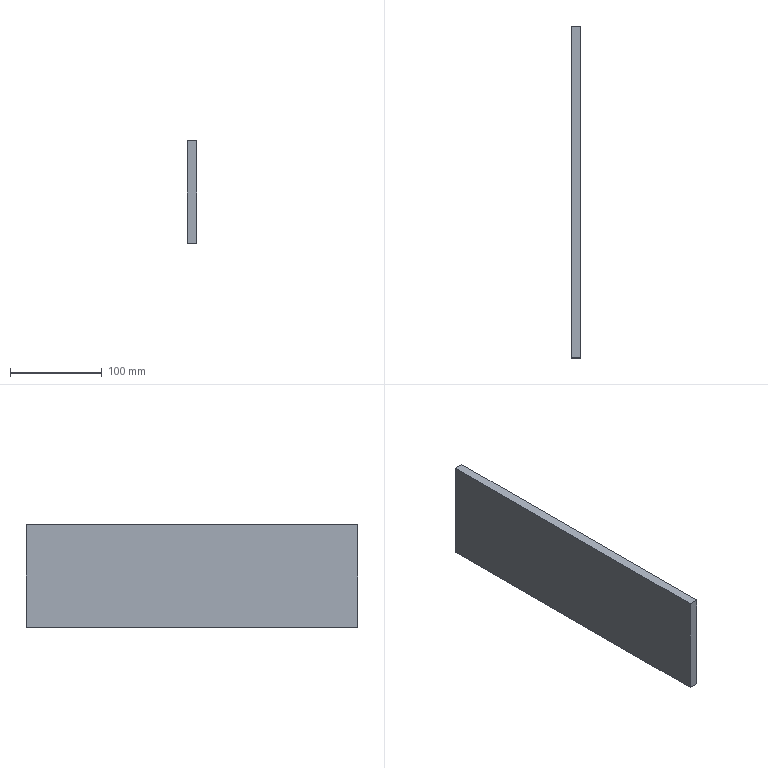Part | STEP file | Drawer | 1 solid | 6 faces | box 10 x 362 x 112 mm | volume 405440 mm3 | plane 6
STEP:
#1=CARTESIAN_POINT('',(0.,0.,0.));
#2=DIRECTION('',(0.,0.,1.));
#3=DIRECTION('',(1.,0.,0.));
#4=AXIS2_PLACEMENT_3D('',#1,#2,#3);
#5=CARTESIAN_POINT('',(-5.,181.,112.));
#6=VERTEX_POINT('',#5);
#7=CARTESIAN_POINT('',(-5.,-181.,112.));
#8=VERTEX_POINT('',#7);
#9=CARTESIAN_POINT('',(-5.,181.,112.));
#10=DIRECTION('',(0.,-1.,0.));
#11=VECTOR('',#10,1.);
#12=LINE('',#9,#11);
#13=CARTESIAN_POINT('',(-5.,181.,112.));
#14=DIRECTION('',(1.,0.,0.));
#15=DIRECTION('',(0.,0.,-1.));
#16=AXIS2_PLACEMENT_3D('',#13,#14,#15);
#17=PLANE('',#16);
#18=CARTESIAN_POINT('',(0.,0.));
#19=DIRECTION('',(0.,-1.));
#20=VECTOR('',#19,1.);
#21=LINE('',#18,#20);
#22=(GEOMETRIC_REPRESENTATION_CONTEXT(2)PARAMETRIC_REPRESENTATION_CONTEXT()REPRESENTATION_CONTEXT('',''));
#23=DEFINITIONAL_REPRESENTATION('',(#21),#22);
#24=PCURVE('',#17,#23);
#25=CARTESIAN_POINT('',(5.,181.,112.));
#26=DIRECTION('',(0.,0.,-1.));
#27=DIRECTION('',(-1.,0.,0.));
#28=AXIS2_PLACEMENT_3D('',#25,#26,#27);
#29=PLANE('',#28);
#30=CARTESIAN_POINT('',(10.,0.));
#31=DIRECTION('',(0.,-1.));
#32=VECTOR('',#31,1.);
#33=LINE('',#30,#32);
#34=(GEOMETRIC_REPRESENTATION_CONTEXT(2)PARAMETRIC_REPRESENTATION_CONTEXT()REPRESENTATION_CONTEXT('',''));
#35=DEFINITIONAL_REPRESENTATION('',(#33),#34);
#36=PCURVE('',#29,#35);
#37=SURFACE_CURVE('',#12,(#24,#36),.PCURVE_S1.);
#38=EDGE_CURVE('',#6,#8,#37,.T.);
#39=ORIENTED_EDGE('',*,*,#38,.T.);
#40=CARTESIAN_POINT('',(-5.,-181.,0.));
#41=VERTEX_POINT('',#40);
#42=CARTESIAN_POINT('',(-5.,-181.,112.));
#43=DIRECTION('',(0.,0.,-1.));
#44=VECTOR('',#43,1.);
#45=LINE('',#42,#44);
#46=CARTESIAN_POINT('',(0.,-362.));
#47=DIRECTION('',(1.,0.));
#48=VECTOR('',#47,1.);
#49=LINE('',#46,#48);
#50=(GEOMETRIC_REPRESENTATION_CONTEXT(2)PARAMETRIC_REPRESENTATION_CONTEXT()REPRESENTATION_CONTEXT('',''));
#51=DEFINITIONAL_REPRESENTATION('',(#49),#50);
#52=PCURVE('',#17,#51);
#53=CARTESIAN_POINT('',(0.,-181.,56.));
#54=DIRECTION('',(0.,1.,0.));
#55=DIRECTION('',(0.,0.,1.));
#56=AXIS2_PLACEMENT_3D('',#53,#54,#55);
#57=PLANE('',#56);
#58=CARTESIAN_POINT('',(56.,-5.));
#59=DIRECTION('',(-1.,0.));
#60=VECTOR('',#59,1.);
#61=LINE('',#58,#60);
#62=(GEOMETRIC_REPRESENTATION_CONTEXT(2)PARAMETRIC_REPRESENTATION_CONTEXT()REPRESENTATION_CONTEXT('',''));
#63=DEFINITIONAL_REPRESENTATION('',(#61),#62);
#64=PCURVE('',#57,#63);
#65=SURFACE_CURVE('',#45,(#52,#64),.PCURVE_S1.);
#66=EDGE_CURVE('',#8,#41,#65,.T.);
#67=ORIENTED_EDGE('',*,*,#66,.T.);
#68=CARTESIAN_POINT('',(-5.,181.,0.));
#69=VERTEX_POINT('',#68);
#70=CARTESIAN_POINT('',(-5.,181.,0.));
#71=DIRECTION('',(0.,-1.,0.));
#72=VECTOR('',#71,1.);
#73=LINE('',#70,#72);
#74=CARTESIAN_POINT('',(112.,0.));
#75=DIRECTION('',(0.,-1.));
#76=VECTOR('',#75,1.);
#77=LINE('',#74,#76);
#78=(GEOMETRIC_REPRESENTATION_CONTEXT(2)PARAMETRIC_REPRESENTATION_CONTEXT()REPRESENTATION_CONTEXT('',''));
#79=DEFINITIONAL_REPRESENTATION('',(#77),#78);
#80=PCURVE('',#17,#79);
#81=CARTESIAN_POINT('',(-5.,181.,0.));
#82=DIRECTION('',(0.,0.,1.));
#83=DIRECTION('',(1.,0.,0.));
#84=AXIS2_PLACEMENT_3D('',#81,#82,#83);
#85=PLANE('',#84);
#86=CARTESIAN_POINT('',(0.,0.));
#87=DIRECTION('',(0.,-1.));
#88=VECTOR('',#87,1.);
#89=LINE('',#86,#88);
#90=(GEOMETRIC_REPRESENTATION_CONTEXT(2)PARAMETRIC_REPRESENTATION_CONTEXT()REPRESENTATION_CONTEXT('',''));
#91=DEFINITIONAL_REPRESENTATION('',(#89),#90);
#92=PCURVE('',#85,#91);
#93=SURFACE_CURVE('',#73,(#80,#92),.PCURVE_S1.);
#94=EDGE_CURVE('',#69,#41,#93,.T.);
#95=ORIENTED_EDGE('',*,*,#94,.F.);
#96=CARTESIAN_POINT('',(-5.,181.,112.));
#97=DIRECTION('',(0.,0.,-1.));
#98=VECTOR('',#97,1.);
#99=LINE('',#96,#98);
#100=CARTESIAN_POINT('',(0.,0.));
#101=DIRECTION('',(1.,0.));
#102=VECTOR('',#101,1.);
#103=LINE('',#100,#102);
#104=(GEOMETRIC_REPRESENTATION_CONTEXT(2)PARAMETRIC_REPRESENTATION_CONTEXT()REPRESENTATION_CONTEXT('',''));
#105=DEFINITIONAL_REPRESENTATION('',(#103),#104);
#106=PCURVE('',#17,#105);
#107=CARTESIAN_POINT('',(0.,181.,56.));
#108=DIRECTION('',(0.,1.,0.));
#109=DIRECTION('',(0.,0.,1.));
#110=AXIS2_PLACEMENT_3D('',#107,#108,#109);
#111=PLANE('',#110);
#112=CARTESIAN_POINT('',(56.,-5.));
#113=DIRECTION('',(-1.,0.));
#114=VECTOR('',#113,1.);
#115=LINE('',#112,#114);
#116=(GEOMETRIC_REPRESENTATION_CONTEXT(2)PARAMETRIC_REPRESENTATION_CONTEXT()REPRESENTATION_CONTEXT('',''));
#117=DEFINITIONAL_REPRESENTATION('',(#115),#116);
#118=PCURVE('',#111,#117);
#119=SURFACE_CURVE('',#99,(#106,#118),.PCURVE_S1.);
#120=EDGE_CURVE('',#6,#69,#119,.T.);
#121=ORIENTED_EDGE('',*,*,#120,.F.);
#122=EDGE_LOOP('',(#39,#67,#95,#121));
#123=FACE_BOUND('',#122,.F.);
#124=ADVANCED_FACE('',(#123),#17,.F.);
#125=ORIENTED_EDGE('',*,*,#94,.T.);
#126=CARTESIAN_POINT('',(5.,-181.,0.));
#127=VERTEX_POINT('',#126);
#128=CARTESIAN_POINT('',(-5.,-181.,0.));
#129=DIRECTION('',(1.,0.,0.));
#130=VECTOR('',#129,1.);
#131=LINE('',#128,#130);
#132=CARTESIAN_POINT('',(0.,-362.));
#133=DIRECTION('',(1.,0.));
#134=VECTOR('',#133,1.);
#135=LINE('',#132,#134);
#136=(GEOMETRIC_REPRESENTATION_CONTEXT(2)PARAMETRIC_REPRESENTATION_CONTEXT()REPRESENTATION_CONTEXT('',''));
#137=DEFINITIONAL_REPRESENTATION('',(#135),#136);
#138=PCURVE('',#85,#137);
#139=CARTESIAN_POINT('',(-56.,-5.));
#140=DIRECTION('',(0.,1.));
#141=VECTOR('',#140,1.);
#142=LINE('',#139,#141);
#143=(GEOMETRIC_REPRESENTATION_CONTEXT(2)PARAMETRIC_REPRESENTATION_CONTEXT()REPRESENTATION_CONTEXT('',''));
#144=DEFINITIONAL_REPRESENTATION('',(#142),#143);
#145=PCURVE('',#57,#144);
#146=SURFACE_CURVE('',#131,(#138,#145),.PCURVE_S1.);
#147=EDGE_CURVE('',#41,#127,#146,.T.);
#148=ORIENTED_EDGE('',*,*,#147,.T.);
#149=CARTESIAN_POINT('',(5.,181.,0.));
#150=VERTEX_POINT('',#149);
#151=CARTESIAN_POINT('',(5.,181.,0.));
#152=DIRECTION('',(0.,-1.,0.));
#153=VECTOR('',#152,1.);
#154=LINE('',#151,#153);
#155=CARTESIAN_POINT('',(10.,0.));
#156=DIRECTION('',(0.,-1.));
#157=VECTOR('',#156,1.);
#158=LINE('',#155,#157);
#159=(GEOMETRIC_REPRESENTATION_CONTEXT(2)PARAMETRIC_REPRESENTATION_CONTEXT()REPRESENTATION_CONTEXT('',''));
#160=DEFINITIONAL_REPRESENTATION('',(#158),#159);
#161=PCURVE('',#85,#160);
#162=CARTESIAN_POINT('',(5.,181.,0.));
#163=DIRECTION('',(-1.,0.,0.));
#164=DIRECTION('',(0.,0.,1.));
#165=AXIS2_PLACEMENT_3D('',#162,#163,#164);
#166=PLANE('',#165);
#167=CARTESIAN_POINT('',(0.,0.));
#168=DIRECTION('',(0.,-1.));
#169=VECTOR('',#168,1.);
#170=LINE('',#167,#169);
#171=(GEOMETRIC_REPRESENTATION_CONTEXT(2)PARAMETRIC_REPRESENTATION_CONTEXT()REPRESENTATION_CONTEXT('',''));
#172=DEFINITIONAL_REPRESENTATION('',(#170),#171);
#173=PCURVE('',#166,#172);
#174=SURFACE_CURVE('',#154,(#161,#173),.PCURVE_S1.);
#175=EDGE_CURVE('',#150,#127,#174,.T.);
#176=ORIENTED_EDGE('',*,*,#175,.F.);
#177=CARTESIAN_POINT('',(-5.,181.,0.));
#178=DIRECTION('',(1.,0.,0.));
#179=VECTOR('',#178,1.);
#180=LINE('',#177,#179);
#181=CARTESIAN_POINT('',(0.,0.));
#182=DIRECTION('',(1.,0.));
#183=VECTOR('',#182,1.);
#184=LINE('',#181,#183);
#185=(GEOMETRIC_REPRESENTATION_CONTEXT(2)PARAMETRIC_REPRESENTATION_CONTEXT()REPRESENTATION_CONTEXT('',''));
#186=DEFINITIONAL_REPRESENTATION('',(#184),#185);
#187=PCURVE('',#85,#186);
#188=CARTESIAN_POINT('',(-56.,-5.));
#189=DIRECTION('',(0.,1.));
#190=VECTOR('',#189,1.);
#191=LINE('',#188,#190);
#192=(GEOMETRIC_REPRESENTATION_CONTEXT(2)PARAMETRIC_REPRESENTATION_CONTEXT()REPRESENTATION_CONTEXT('',''));
#193=DEFINITIONAL_REPRESENTATION('',(#191),#192);
#194=PCURVE('',#111,#193);
#195=SURFACE_CURVE('',#180,(#187,#194),.PCURVE_S1.);
#196=EDGE_CURVE('',#69,#150,#195,.T.);
#197=ORIENTED_EDGE('',*,*,#196,.F.);
#198=EDGE_LOOP('',(#125,#148,#176,#197));
#199=FACE_BOUND('',#198,.F.);
#200=ADVANCED_FACE('',(#199),#85,.F.);
#201=ORIENTED_EDGE('',*,*,#175,.T.);
#202=CARTESIAN_POINT('',(5.,-181.,112.));
#203=VERTEX_POINT('',#202);
#204=CARTESIAN_POINT('',(5.,-181.,0.));
#205=DIRECTION('',(0.,0.,1.));
#206=VECTOR('',#205,1.);
#207=LINE('',#204,#206);
#208=CARTESIAN_POINT('',(0.,-362.));
#209=DIRECTION('',(1.,0.));
#210=VECTOR('',#209,1.);
#211=LINE('',#208,#210);
#212=(GEOMETRIC_REPRESENTATION_CONTEXT(2)PARAMETRIC_REPRESENTATION_CONTEXT()REPRESENTATION_CONTEXT('',''));
#213=DEFINITIONAL_REPRESENTATION('',(#211),#212);
#214=PCURVE('',#166,#213);
#215=CARTESIAN_POINT('',(-56.,5.));
#216=DIRECTION('',(1.,0.));
#217=VECTOR('',#216,1.);
#218=LINE('',#215,#217);
#219=(GEOMETRIC_REPRESENTATION_CONTEXT(2)PARAMETRIC_REPRESENTATION_CONTEXT()REPRESENTATION_CONTEXT('',''));
#220=DEFINITIONAL_REPRESENTATION('',(#218),#219);
#221=PCURVE('',#57,#220);
#222=SURFACE_CURVE('',#207,(#214,#221),.PCURVE_S1.);
#223=EDGE_CURVE('',#127,#203,#222,.T.);
#224=ORIENTED_EDGE('',*,*,#223,.T.);
#225=CARTESIAN_POINT('',(5.,181.,112.));
#226=VERTEX_POINT('',#225);
#227=CARTESIAN_POINT('',(5.,181.,112.));
#228=DIRECTION('',(0.,-1.,0.));
#229=VECTOR('',#228,1.);
#230=LINE('',#227,#229);
#231=CARTESIAN_POINT('',(112.,0.));
#232=DIRECTION('',(0.,-1.));
#233=VECTOR('',#232,1.);
#234=LINE('',#231,#233);
#235=(GEOMETRIC_REPRESENTATION_CONTEXT(2)PARAMETRIC_REPRESENTATION_CONTEXT()REPRESENTATION_CONTEXT('',''));
#236=DEFINITIONAL_REPRESENTATION('',(#234),#235);
#237=PCURVE('',#166,#236);
#238=CARTESIAN_POINT('',(0.,0.));
#239=DIRECTION('',(0.,-1.));
#240=VECTOR('',#239,1.);
#241=LINE('',#238,#240);
#242=(GEOMETRIC_REPRESENTATION_CONTEXT(2)PARAMETRIC_REPRESENTATION_CONTEXT()REPRESENTATION_CONTEXT('',''));
#243=DEFINITIONAL_REPRESENTATION('',(#241),#242);
#244=PCURVE('',#29,#243);
#245=SURFACE_CURVE('',#230,(#237,#244),.PCURVE_S1.);
#246=EDGE_CURVE('',#226,#203,#245,.T.);
#247=ORIENTED_EDGE('',*,*,#246,.F.);
#248=CARTESIAN_POINT('',(5.,181.,0.));
#249=DIRECTION('',(0.,0.,1.));
#250=VECTOR('',#249,1.);
#251=LINE('',#248,#250);
#252=CARTESIAN_POINT('',(0.,0.));
#253=DIRECTION('',(1.,0.));
#254=VECTOR('',#253,1.);
#255=LINE('',#252,#254);
#256=(GEOMETRIC_REPRESENTATION_CONTEXT(2)PARAMETRIC_REPRESENTATION_CONTEXT()REPRESENTATION_CONTEXT('',''));
#257=DEFINITIONAL_REPRESENTATION('',(#255),#256);
#258=PCURVE('',#166,#257);
#259=CARTESIAN_POINT('',(-56.,5.));
#260=DIRECTION('',(1.,0.));
#261=VECTOR('',#260,1.);
#262=LINE('',#259,#261);
#263=(GEOMETRIC_REPRESENTATION_CONTEXT(2)PARAMETRIC_REPRESENTATION_CONTEXT()REPRESENTATION_CONTEXT('',''));
#264=DEFINITIONAL_REPRESENTATION('',(#262),#263);
#265=PCURVE('',#111,#264);
#266=SURFACE_CURVE('',#251,(#258,#265),.PCURVE_S1.);
#267=EDGE_CURVE('',#150,#226,#266,.T.);
#268=ORIENTED_EDGE('',*,*,#267,.F.);
#269=EDGE_LOOP('',(#201,#224,#247,#268));
#270=FACE_BOUND('',#269,.F.);
#271=ADVANCED_FACE('',(#270),#166,.F.);
#272=ORIENTED_EDGE('',*,*,#246,.T.);
#273=CARTESIAN_POINT('',(5.,-181.,112.));
#274=DIRECTION('',(-1.,0.,0.));
#275=VECTOR('',#274,1.);
#276=LINE('',#273,#275);
#277=CARTESIAN_POINT('',(0.,-362.));
#278=DIRECTION('',(1.,0.));
#279=VECTOR('',#278,1.);
#280=LINE('',#277,#279);
#281=(GEOMETRIC_REPRESENTATION_CONTEXT(2)PARAMETRIC_REPRESENTATION_CONTEXT()REPRESENTATION_CONTEXT('',''));
#282=DEFINITIONAL_REPRESENTATION('',(#280),#281);
#283=PCURVE('',#29,#282);
#284=CARTESIAN_POINT('',(56.,5.));
#285=DIRECTION('',(0.,-1.));
#286=VECTOR('',#285,1.);
#287=LINE('',#284,#286);
#288=(GEOMETRIC_REPRESENTATION_CONTEXT(2)PARAMETRIC_REPRESENTATION_CONTEXT()REPRESENTATION_CONTEXT('',''));
#289=DEFINITIONAL_REPRESENTATION('',(#287),#288);
#290=PCURVE('',#57,#289);
#291=SURFACE_CURVE('',#276,(#283,#290),.PCURVE_S1.);
#292=EDGE_CURVE('',#203,#8,#291,.T.);
#293=ORIENTED_EDGE('',*,*,#292,.T.);
#294=ORIENTED_EDGE('',*,*,#38,.F.);
#295=CARTESIAN_POINT('',(5.,181.,112.));
#296=DIRECTION('',(-1.,0.,0.));
#297=VECTOR('',#296,1.);
#298=LINE('',#295,#297);
#299=CARTESIAN_POINT('',(0.,0.));
#300=DIRECTION('',(1.,0.));
#301=VECTOR('',#300,1.);
#302=LINE('',#299,#301);
#303=(GEOMETRIC_REPRESENTATION_CONTEXT(2)PARAMETRIC_REPRESENTATION_CONTEXT()REPRESENTATION_CONTEXT('',''));
#304=DEFINITIONAL_REPRESENTATION('',(#302),#303);
#305=PCURVE('',#29,#304);
#306=CARTESIAN_POINT('',(56.,5.));
#307=DIRECTION('',(0.,-1.));
#308=VECTOR('',#307,1.);
#309=LINE('',#306,#308);
#310=(GEOMETRIC_REPRESENTATION_CONTEXT(2)PARAMETRIC_REPRESENTATION_CONTEXT()REPRESENTATION_CONTEXT('',''));
#311=DEFINITIONAL_REPRESENTATION('',(#309),#310);
#312=PCURVE('',#111,#311);
#313=SURFACE_CURVE('',#298,(#305,#312),.PCURVE_S1.);
#314=EDGE_CURVE('',#226,#6,#313,.T.);
#315=ORIENTED_EDGE('',*,*,#314,.F.);
#316=EDGE_LOOP('',(#272,#293,#294,#315));
#317=FACE_BOUND('',#316,.F.);
#318=ADVANCED_FACE('',(#317),#29,.F.);
#319=ORIENTED_EDGE('',*,*,#120,.T.);
#320=ORIENTED_EDGE('',*,*,#196,.T.);
#321=ORIENTED_EDGE('',*,*,#267,.T.);
#322=ORIENTED_EDGE('',*,*,#314,.T.);
#323=EDGE_LOOP('',(#319,#320,#321,#322));
#324=FACE_BOUND('',#323,.F.);
#325=ADVANCED_FACE('',(#324),#111,.T.);
#326=ORIENTED_EDGE('',*,*,#66,.T.);
#327=ORIENTED_EDGE('',*,*,#147,.T.);
#328=ORIENTED_EDGE('',*,*,#223,.T.);
#329=ORIENTED_EDGE('',*,*,#292,.T.);
#330=EDGE_LOOP('',(#326,#327,#328,#329));
#331=FACE_BOUND('',#330,.T.);
#332=ADVANCED_FACE('',(#331),#57,.F.);
#333=CLOSED_SHELL('',(#124,#200,#271,#318,#325,#332));
#334=MANIFOLD_SOLID_BREP('',#333);
#335=(LENGTH_UNIT()NAMED_UNIT(*)SI_UNIT(.MILLI.,.METRE.));
#336=UNCERTAINTY_MEASURE_WITH_UNIT(LENGTH_MEASURE(0.0000001),#335,'','');
#337=(NAMED_UNIT(*)PLANE_ANGLE_UNIT()SI_UNIT($,.RADIAN.));
#338=(NAMED_UNIT(*)SI_UNIT($,.STERADIAN.)SOLID_ANGLE_UNIT());
#339=(GEOMETRIC_REPRESENTATION_CONTEXT(3)GLOBAL_UNCERTAINTY_ASSIGNED_CONTEXT((#336))GLOBAL_UNIT_ASSIGNED_CONTEXT((#335,#337,#338))REPRESENTATION_CONTEXT('',''));
#340=ADVANCED_BREP_SHAPE_REPRESENTATION('',(#4,#334),#339);